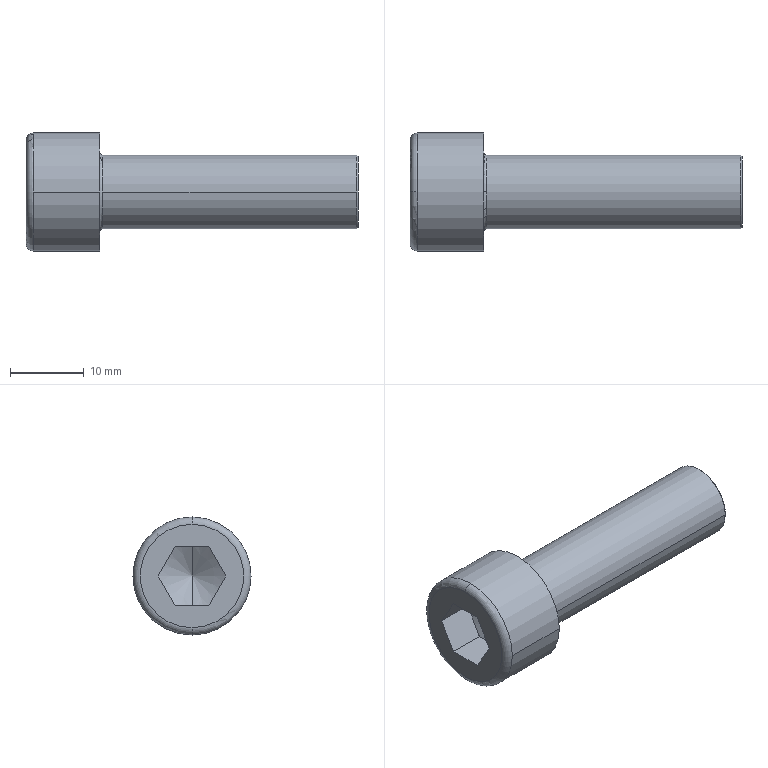Part | SolidWorks | features BaseBody 1 | 1 solid | 27 faces | box 45 x 16 x 16 mm | volume 4420 mm3 | plane 15 | cylinder 4 | cone 4 | torus 4 | commonest cylinder face diameters 10 x2 16 x2
STEP:
#1=CARTESIAN_POINT('',(34.8,0.,5.));
#2=VERTEX_POINT('',#1);
#3=CARTESIAN_POINT('',(34.8,5.,0.));
#4=VERTEX_POINT('',#3);
#5=CARTESIAN_POINT('',(34.8,0.,0.));
#6=DIRECTION('',(-1.,0.,0.));
#7=DIRECTION('',(0.,-1.,0.));
#8=AXIS2_PLACEMENT_3D('',#5,#6,#7);
#9=CIRCLE('',#8,5.);
#10=EDGE_CURVE('',#2,#4,#9,.T.);
#11=ORIENTED_EDGE('',*,*,#10,.T.);
#12=CARTESIAN_POINT('',(0.4,5.,0.));
#13=VERTEX_POINT('',#12);
#14=CARTESIAN_POINT('',(-2.359,5.,0.));
#15=DIRECTION('',(-1.,0.,0.));
#16=VECTOR('',#15,1000.);
#17=LINE('',#14,#16);
#18=EDGE_CURVE('',#4,#13,#17,.T.);
#19=ORIENTED_EDGE('',*,*,#18,.T.);
#20=CARTESIAN_POINT('',(0.4,0.,5.));
#21=VERTEX_POINT('',#20);
#22=CARTESIAN_POINT('',(0.4,0.,0.));
#23=DIRECTION('',(1.,0.,0.));
#24=DIRECTION('',(0.,-1.,0.));
#25=AXIS2_PLACEMENT_3D('',#22,#23,#24);
#26=CIRCLE('',#25,5.);
#27=EDGE_CURVE('',#13,#21,#26,.T.);
#28=ORIENTED_EDGE('',*,*,#27,.T.);
#29=CARTESIAN_POINT('',(0.4,-5.,0.));
#30=VERTEX_POINT('',#29);
#31=CARTESIAN_POINT('',(0.4,0.,0.));
#32=DIRECTION('',(1.,0.,0.));
#33=DIRECTION('',(0.,-1.,0.));
#34=AXIS2_PLACEMENT_3D('',#31,#32,#33);
#35=CIRCLE('',#34,5.);
#36=EDGE_CURVE('',#21,#30,#35,.T.);
#37=ORIENTED_EDGE('',*,*,#36,.T.);
#38=CARTESIAN_POINT('',(34.8,-5.,0.));
#39=VERTEX_POINT('',#38);
#40=CARTESIAN_POINT('',(-2.359,-5.,0.));
#41=DIRECTION('',(-1.,0.,0.));
#42=VECTOR('',#41,1000.);
#43=LINE('',#40,#42);
#44=EDGE_CURVE('',#39,#30,#43,.T.);
#45=ORIENTED_EDGE('',*,*,#44,.F.);
#46=CARTESIAN_POINT('',(34.8,0.,0.));
#47=DIRECTION('',(-1.,0.,0.));
#48=DIRECTION('',(0.,-1.,0.));
#49=AXIS2_PLACEMENT_3D('',#46,#47,#48);
#50=CIRCLE('',#49,5.);
#51=EDGE_CURVE('',#39,#2,#50,.T.);
#52=ORIENTED_EDGE('',*,*,#51,.T.);
#53=EDGE_LOOP('',(#11,#19,#28,#37,#45,#52));
#54=FACE_OUTER_BOUND('',#53,.T.);
#55=CARTESIAN_POINT('',(-2.359,0.,0.));
#56=DIRECTION('',(-1.,0.,0.));
#57=DIRECTION('',(0.,-1.,0.));
#58=AXIS2_PLACEMENT_3D('',#55,#56,#57);
#59=CYLINDRICAL_SURFACE('',#58,5.);
#60=ADVANCED_FACE('',(#54),#59,.T.);
#61=CARTESIAN_POINT('',(35.,0.,4.8));
#62=VERTEX_POINT('',#61);
#63=CARTESIAN_POINT('',(35.,0.,-4.8));
#64=VERTEX_POINT('',#63);
#65=CARTESIAN_POINT('',(35.,0.,0.));
#66=DIRECTION('',(-1.,0.,0.));
#67=DIRECTION('',(0.,0.,1.));
#68=AXIS2_PLACEMENT_3D('',#65,#66,#67);
#69=CIRCLE('',#68,4.8);
#70=EDGE_CURVE('',#62,#64,#69,.T.);
#71=ORIENTED_EDGE('',*,*,#70,.T.);
#72=CARTESIAN_POINT('',(34.8,0.,-5.));
#73=VERTEX_POINT('',#72);
#74=CARTESIAN_POINT('',(34.8,0.,-5.));
#75=DIRECTION('',(-0.7071,0.,-0.7071));
#76=VECTOR('',#75,1000.);
#77=LINE('',#74,#76);
#78=EDGE_CURVE('',#64,#73,#77,.T.);
#79=ORIENTED_EDGE('',*,*,#78,.T.);
#80=CARTESIAN_POINT('',(34.8,0.,0.));
#81=DIRECTION('',(-1.,0.,0.));
#82=DIRECTION('',(0.,-1.,0.));
#83=AXIS2_PLACEMENT_3D('',#80,#81,#82);
#84=CIRCLE('',#83,5.);
#85=EDGE_CURVE('',#4,#73,#84,.T.);
#86=ORIENTED_EDGE('',*,*,#85,.F.);
#87=ORIENTED_EDGE('',*,*,#10,.F.);
#88=CARTESIAN_POINT('',(34.8,0.,5.));
#89=DIRECTION('',(-0.7071,0.,0.7071));
#90=VECTOR('',#89,1000.);
#91=LINE('',#88,#90);
#92=EDGE_CURVE('',#62,#2,#91,.T.);
#93=ORIENTED_EDGE('',*,*,#92,.F.);
#94=EDGE_LOOP('',(#71,#79,#86,#87,#93));
#95=FACE_OUTER_BOUND('',#94,.T.);
#96=CARTESIAN_POINT('',(34.8,0.,0.));
#97=DIRECTION('',(-1.,0.,0.));
#98=DIRECTION('',(0.,0.,1.));
#99=AXIS2_PLACEMENT_3D('',#96,#97,#98);
#100=CONICAL_SURFACE('',#99,5.,0.7854);
#101=ADVANCED_FACE('',(#95),#100,.T.);
#102=CARTESIAN_POINT('',(0.,0.,-5.4));
#103=VERTEX_POINT('',#102);
#104=CARTESIAN_POINT('',(0.,0.,5.4));
#105=VERTEX_POINT('',#104);
#106=CARTESIAN_POINT('',(0.,0.,0.));
#107=DIRECTION('',(-1.,0.,0.));
#108=DIRECTION('',(0.,0.,1.));
#109=AXIS2_PLACEMENT_3D('',#106,#107,#108);
#110=CIRCLE('',#109,5.4);
#111=EDGE_CURVE('',#103,#105,#110,.T.);
#112=ORIENTED_EDGE('',*,*,#111,.F.);
#113=CARTESIAN_POINT('',(0.4,0.,-5.));
#114=VERTEX_POINT('',#113);
#115=CARTESIAN_POINT('',(0.4,0.,-5.4));
#116=DIRECTION('',(0.,1.,0.));
#117=DIRECTION('',(0.,0.,1.));
#118=AXIS2_PLACEMENT_3D('',#115,#116,#117);
#119=CIRCLE('',#118,0.4);
#120=EDGE_CURVE('',#103,#114,#119,.T.);
#121=ORIENTED_EDGE('',*,*,#120,.T.);
#122=CARTESIAN_POINT('',(0.4,0.,0.));
#123=DIRECTION('',(1.,0.,0.));
#124=DIRECTION('',(0.,-1.,0.));
#125=AXIS2_PLACEMENT_3D('',#122,#123,#124);
#126=CIRCLE('',#125,5.);
#127=EDGE_CURVE('',#30,#114,#126,.T.);
#128=ORIENTED_EDGE('',*,*,#127,.F.);
#129=ORIENTED_EDGE('',*,*,#36,.F.);
#130=CARTESIAN_POINT('',(0.4,0.,5.4));
#131=DIRECTION('',(0.,-1.,0.));
#132=DIRECTION('',(1.,0.,0.));
#133=AXIS2_PLACEMENT_3D('',#130,#131,#132);
#134=CIRCLE('',#133,0.4);
#135=EDGE_CURVE('',#105,#21,#134,.T.);
#136=ORIENTED_EDGE('',*,*,#135,.F.);
#137=EDGE_LOOP('',(#112,#121,#128,#129,#136));
#138=FACE_OUTER_BOUND('',#137,.T.);
#139=CARTESIAN_POINT('',(0.4,0.,0.));
#140=DIRECTION('',(-1.,0.,0.));
#141=DIRECTION('',(0.,0.,1.));
#142=AXIS2_PLACEMENT_3D('',#139,#140,#141);
#143=TOROIDAL_SURFACE('',#142,5.4,0.4);
#144=ADVANCED_FACE('',(#138),#143,.F.);
#145=CARTESIAN_POINT('',(0.,-8.,0.));
#146=VERTEX_POINT('',#145);
#147=CARTESIAN_POINT('',(0.,8.,0.));
#148=VERTEX_POINT('',#147);
#149=CARTESIAN_POINT('',(0.,0.,0.));
#150=DIRECTION('',(-1.,0.,0.));
#151=DIRECTION('',(0.,-1.,0.));
#152=AXIS2_PLACEMENT_3D('',#149,#150,#151);
#153=CIRCLE('',#152,8.);
#154=EDGE_CURVE('',#146,#148,#153,.T.);
#155=ORIENTED_EDGE('',*,*,#154,.T.);
#156=CARTESIAN_POINT('',(-9.,8.,0.));
#157=VERTEX_POINT('',#156);
#158=CARTESIAN_POINT('',(-2.359,8.,0.));
#159=DIRECTION('',(-1.,0.,0.));
#160=VECTOR('',#159,1000.);
#161=LINE('',#158,#160);
#162=EDGE_CURVE('',#148,#157,#161,.T.);
#163=ORIENTED_EDGE('',*,*,#162,.T.);
#164=CARTESIAN_POINT('',(-9.,0.,8.));
#165=VERTEX_POINT('',#164);
#166=CARTESIAN_POINT('',(-9.,0.,0.));
#167=DIRECTION('',(1.,0.,0.));
#168=DIRECTION('',(0.,-1.,0.));
#169=AXIS2_PLACEMENT_3D('',#166,#167,#168);
#170=CIRCLE('',#169,8.);
#171=EDGE_CURVE('',#157,#165,#170,.T.);
#172=ORIENTED_EDGE('',*,*,#171,.T.);
#173=CARTESIAN_POINT('',(-9.,-8.,0.));
#174=VERTEX_POINT('',#173);
#175=CARTESIAN_POINT('',(-9.,0.,0.));
#176=DIRECTION('',(1.,0.,0.));
#177=DIRECTION('',(0.,-1.,0.));
#178=AXIS2_PLACEMENT_3D('',#175,#176,#177);
#179=CIRCLE('',#178,8.);
#180=EDGE_CURVE('',#165,#174,#179,.T.);
#181=ORIENTED_EDGE('',*,*,#180,.T.);
#182=CARTESIAN_POINT('',(-2.359,-8.,0.));
#183=DIRECTION('',(-1.,0.,0.));
#184=VECTOR('',#183,1000.);
#185=LINE('',#182,#184);
#186=EDGE_CURVE('',#146,#174,#185,.T.);
#187=ORIENTED_EDGE('',*,*,#186,.F.);
#188=EDGE_LOOP('',(#155,#163,#172,#181,#187));
#189=FACE_OUTER_BOUND('',#188,.T.);
#190=CARTESIAN_POINT('',(-2.359,0.,0.));
#191=DIRECTION('',(-1.,0.,0.));
#192=DIRECTION('',(0.,-1.,0.));
#193=AXIS2_PLACEMENT_3D('',#190,#191,#192);
#194=CYLINDRICAL_SURFACE('',#193,8.);
#195=ADVANCED_FACE('',(#189),#194,.T.);
#196=CARTESIAN_POINT('',(-9.,0.,-8.));
#197=VERTEX_POINT('',#196);
#198=CARTESIAN_POINT('',(-9.,0.,0.));
#199=DIRECTION('',(1.,0.,0.));
#200=DIRECTION('',(0.,-1.,0.));
#201=AXIS2_PLACEMENT_3D('',#198,#199,#200);
#202=CIRCLE('',#201,8.);
#203=EDGE_CURVE('',#197,#157,#202,.T.);
#204=ORIENTED_EDGE('',*,*,#203,.F.);
#205=CARTESIAN_POINT('',(-10.,0.,-7.));
#206=VERTEX_POINT('',#205);
#207=CARTESIAN_POINT('',(-9.,0.,-7.));
#208=DIRECTION('',(0.,1.,0.));
#209=DIRECTION('',(0.,0.,1.));
#210=AXIS2_PLACEMENT_3D('',#207,#208,#209);
#211=CIRCLE('',#210,1.);
#212=EDGE_CURVE('',#197,#206,#211,.T.);
#213=ORIENTED_EDGE('',*,*,#212,.T.);
#214=CARTESIAN_POINT('',(-10.,0.,7.));
#215=VERTEX_POINT('',#214);
#216=CARTESIAN_POINT('',(-10.,0.,0.));
#217=DIRECTION('',(1.,0.,0.));
#218=DIRECTION('',(0.,0.,1.));
#219=AXIS2_PLACEMENT_3D('',#216,#217,#218);
#220=CIRCLE('',#219,7.);
#221=EDGE_CURVE('',#206,#215,#220,.T.);
#222=ORIENTED_EDGE('',*,*,#221,.T.);
#223=CARTESIAN_POINT('',(-9.,0.,7.));
#224=DIRECTION('',(0.,-1.,0.));
#225=DIRECTION('',(0.,0.,-1.));
#226=AXIS2_PLACEMENT_3D('',#223,#224,#225);
#227=CIRCLE('',#226,1.);
#228=EDGE_CURVE('',#165,#215,#227,.T.);
#229=ORIENTED_EDGE('',*,*,#228,.F.);
#230=ORIENTED_EDGE('',*,*,#171,.F.);
#231=EDGE_LOOP('',(#204,#213,#222,#229,#230));
#232=FACE_OUTER_BOUND('',#231,.T.);
#233=CARTESIAN_POINT('',(-9.,0.,0.));
#234=DIRECTION('',(-1.,0.,0.));
#235=DIRECTION('',(0.,0.,1.));
#236=AXIS2_PLACEMENT_3D('',#233,#234,#235);
#237=TOROIDAL_SURFACE('',#236,7.,1.);
#238=ADVANCED_FACE('',(#232),#237,.T.);
#239=CARTESIAN_POINT('',(-2.359,0.,0.));
#240=VERTEX_POINT('',#239);
#241=CARTESIAN_POINT('',(-5.,0.,4.574));
#242=VERTEX_POINT('',#241);
#243=CARTESIAN_POINT('',(-5.,0.,4.575));
#244=DIRECTION('',(-0.5,0.,0.866));
#245=VECTOR('',#244,1000.);
#246=LINE('',#243,#245);
#247=EDGE_CURVE('',#240,#242,#246,.T.);
#248=ORIENTED_EDGE('',*,*,#247,.F.);
#249=CARTESIAN_POINT('',(-5.,0.,-4.575));
#250=VERTEX_POINT('',#249);
#251=CARTESIAN_POINT('',(-5.,0.,-4.575));
#252=DIRECTION('',(-0.5,0.,-0.866));
#253=VECTOR('',#252,1000.);
#254=LINE('',#251,#253);
#255=EDGE_CURVE('',#240,#250,#254,.T.);
#256=ORIENTED_EDGE('',*,*,#255,.T.);
#257=CARTESIAN_POINT('',(-5.,-2.287,-3.962));
#258=VERTEX_POINT('',#257);
#259=CARTESIAN_POINT('',(-5.,0.,0.));
#260=DIRECTION('',(-1.,0.,0.));
#261=DIRECTION('',(0.,0.,1.));
#262=AXIS2_PLACEMENT_3D('',#259,#260,#261);
#263=CIRCLE('',#262,4.574);
#264=EDGE_CURVE('',#250,#258,#263,.T.);
#265=ORIENTED_EDGE('',*,*,#264,.T.);
#266=CARTESIAN_POINT('',(-5.,-4.575,0.));
#267=VERTEX_POINT('',#266);
#268=CARTESIAN_POINT('',(-5.,0.,0.));
#269=DIRECTION('',(-1.,0.,0.));
#270=DIRECTION('',(0.,0.,1.));
#271=AXIS2_PLACEMENT_3D('',#268,#269,#270);
#272=CIRCLE('',#271,4.575);
#273=EDGE_CURVE('',#258,#267,#272,.T.);
#274=ORIENTED_EDGE('',*,*,#273,.T.);
#275=CARTESIAN_POINT('',(-5.,-2.287,3.962));
#276=VERTEX_POINT('',#275);
#277=CARTESIAN_POINT('',(-5.,0.,0.));
#278=DIRECTION('',(-1.,0.,0.));
#279=DIRECTION('',(0.,0.,1.));
#280=AXIS2_PLACEMENT_3D('',#277,#278,#279);
#281=CIRCLE('',#280,4.574);
#282=EDGE_CURVE('',#267,#276,#281,.T.);
#283=ORIENTED_EDGE('',*,*,#282,.T.);
#284=CARTESIAN_POINT('',(-5.,0.,0.));
#285=DIRECTION('',(-1.,0.,0.));
#286=DIRECTION('',(0.,0.,1.));
#287=AXIS2_PLACEMENT_3D('',#284,#285,#286);
#288=CIRCLE('',#287,4.574);
#289=EDGE_CURVE('',#276,#242,#288,.T.);
#290=ORIENTED_EDGE('',*,*,#289,.T.);
#291=EDGE_LOOP('',(#248,#256,#265,#274,#283,#290));
#292=FACE_OUTER_BOUND('',#291,.T.);
#293=CARTESIAN_POINT('',(-5.,0.,0.));
#294=DIRECTION('',(-1.,0.,0.));
#295=DIRECTION('',(0.,0.,1.));
#296=AXIS2_PLACEMENT_3D('',#293,#294,#295);
#297=CONICAL_SURFACE('',#296,4.575,1.047);
#298=ADVANCED_FACE('',(#292),#297,.F.);
#299=ORIENTED_EDGE('',*,*,#18,.F.);
#300=ORIENTED_EDGE('',*,*,#85,.T.);
#301=CARTESIAN_POINT('',(34.8,0.,0.));
#302=DIRECTION('',(-1.,0.,0.));
#303=DIRECTION('',(0.,-1.,0.));
#304=AXIS2_PLACEMENT_3D('',#301,#302,#303);
#305=CIRCLE('',#304,5.);
#306=EDGE_CURVE('',#73,#39,#305,.T.);
#307=ORIENTED_EDGE('',*,*,#306,.T.);
#308=ORIENTED_EDGE('',*,*,#44,.T.);
#309=ORIENTED_EDGE('',*,*,#127,.T.);
#310=CARTESIAN_POINT('',(0.4,0.,0.));
#311=DIRECTION('',(1.,0.,0.));
#312=DIRECTION('',(0.,-1.,0.));
#313=AXIS2_PLACEMENT_3D('',#310,#311,#312);
#314=CIRCLE('',#313,5.);
#315=EDGE_CURVE('',#114,#13,#314,.T.);
#316=ORIENTED_EDGE('',*,*,#315,.T.);
#317=EDGE_LOOP('',(#299,#300,#307,#308,#309,#316));
#318=FACE_OUTER_BOUND('',#317,.T.);
#319=CARTESIAN_POINT('',(-2.359,0.,0.));
#320=DIRECTION('',(-1.,0.,0.));
#321=DIRECTION('',(0.,-1.,0.));
#322=AXIS2_PLACEMENT_3D('',#319,#320,#321);
#323=CYLINDRICAL_SURFACE('',#322,5.);
#324=ADVANCED_FACE('',(#318),#323,.T.);
#325=ORIENTED_EDGE('',*,*,#78,.F.);
#326=CARTESIAN_POINT('',(35.,0.,0.));
#327=DIRECTION('',(-1.,0.,0.));
#328=DIRECTION('',(0.,0.,1.));
#329=AXIS2_PLACEMENT_3D('',#326,#327,#328);
#330=CIRCLE('',#329,4.8);
#331=EDGE_CURVE('',#64,#62,#330,.T.);
#332=ORIENTED_EDGE('',*,*,#331,.T.);
#333=ORIENTED_EDGE('',*,*,#92,.T.);
#334=ORIENTED_EDGE('',*,*,#51,.F.);
#335=ORIENTED_EDGE('',*,*,#306,.F.);
#336=EDGE_LOOP('',(#325,#332,#333,#334,#335));
#337=FACE_OUTER_BOUND('',#336,.T.);
#338=CARTESIAN_POINT('',(34.8,0.,0.));
#339=DIRECTION('',(-1.,0.,0.));
#340=DIRECTION('',(0.,0.,1.));
#341=AXIS2_PLACEMENT_3D('',#338,#339,#340);
#342=CONICAL_SURFACE('',#341,5.,0.7854);
#343=ADVANCED_FACE('',(#337),#342,.T.);
#344=ORIENTED_EDGE('',*,*,#120,.F.);
#345=CARTESIAN_POINT('',(0.,0.,0.));
#346=DIRECTION('',(-1.,0.,0.));
#347=DIRECTION('',(0.,0.,1.));
#348=AXIS2_PLACEMENT_3D('',#345,#346,#347);
#349=CIRCLE('',#348,5.4);
#350=EDGE_CURVE('',#105,#103,#349,.T.);
#351=ORIENTED_EDGE('',*,*,#350,.F.);
#352=ORIENTED_EDGE('',*,*,#135,.T.);
#353=ORIENTED_EDGE('',*,*,#27,.F.);
#354=ORIENTED_EDGE('',*,*,#315,.F.);
#355=EDGE_LOOP('',(#344,#351,#352,#353,#354));
#356=FACE_OUTER_BOUND('',#355,.T.);
#357=CARTESIAN_POINT('',(0.4,0.,0.));
#358=DIRECTION('',(-1.,0.,0.));
#359=DIRECTION('',(0.,0.,1.));
#360=AXIS2_PLACEMENT_3D('',#357,#358,#359);
#361=TOROIDAL_SURFACE('',#360,5.4,0.4);
#362=ADVANCED_FACE('',(#356),#361,.F.);
#363=ORIENTED_EDGE('',*,*,#70,.F.);
#364=ORIENTED_EDGE('',*,*,#331,.F.);
#365=EDGE_LOOP('',(#363,#364));
#366=FACE_OUTER_BOUND('',#365,.T.);
#367=CARTESIAN_POINT('',(35.,4.8,0.));
#368=DIRECTION('',(-1.,0.,0.));
#369=DIRECTION('',(0.,-1.,0.));
#370=AXIS2_PLACEMENT_3D('',#367,#368,#369);
#371=PLANE('',#370);
#372=ADVANCED_FACE('',(#366),#371,.F.);
#373=ORIENTED_EDGE('',*,*,#154,.F.);
#374=CARTESIAN_POINT('',(0.,0.,0.));
#375=DIRECTION('',(-1.,0.,0.));
#376=DIRECTION('',(0.,-1.,0.));
#377=AXIS2_PLACEMENT_3D('',#374,#375,#376);
#378=CIRCLE('',#377,8.);
#379=EDGE_CURVE('',#148,#146,#378,.T.);
#380=ORIENTED_EDGE('',*,*,#379,.F.);
#381=EDGE_LOOP('',(#373,#380));
#382=FACE_OUTER_BOUND('',#381,.T.);
#383=ORIENTED_EDGE('',*,*,#350,.T.);
#384=ORIENTED_EDGE('',*,*,#111,.T.);
#385=EDGE_LOOP('',(#383,#384));
#386=FACE_BOUND('',#385,.T.);
#387=CARTESIAN_POINT('',(0.,8.,0.));
#388=DIRECTION('',(-1.,0.,0.));
#389=DIRECTION('',(0.,-1.,0.));
#390=AXIS2_PLACEMENT_3D('',#387,#388,#389);
#391=PLANE('',#390);
#392=ADVANCED_FACE('',(#382,#386),#391,.F.);
#393=ORIENTED_EDGE('',*,*,#162,.F.);
#394=ORIENTED_EDGE('',*,*,#379,.T.);
#395=ORIENTED_EDGE('',*,*,#186,.T.);
#396=CARTESIAN_POINT('',(-9.,0.,0.));
#397=DIRECTION('',(1.,0.,0.));
#398=DIRECTION('',(0.,-1.,0.));
#399=AXIS2_PLACEMENT_3D('',#396,#397,#398);
#400=CIRCLE('',#399,8.);
#401=EDGE_CURVE('',#174,#197,#400,.T.);
#402=ORIENTED_EDGE('',*,*,#401,.T.);
#403=ORIENTED_EDGE('',*,*,#203,.T.);
#404=EDGE_LOOP('',(#393,#394,#395,#402,#403));
#405=FACE_OUTER_BOUND('',#404,.T.);
#406=CARTESIAN_POINT('',(-2.359,0.,0.));
#407=DIRECTION('',(-1.,0.,0.));
#408=DIRECTION('',(0.,-1.,0.));
#409=AXIS2_PLACEMENT_3D('',#406,#407,#408);
#410=CYLINDRICAL_SURFACE('',#409,8.);
#411=ADVANCED_FACE('',(#405),#410,.T.);
#412=ORIENTED_EDGE('',*,*,#212,.F.);
#413=ORIENTED_EDGE('',*,*,#401,.F.);
#414=ORIENTED_EDGE('',*,*,#180,.F.);
#415=ORIENTED_EDGE('',*,*,#228,.T.);
#416=CARTESIAN_POINT('',(-10.,0.,0.));
#417=DIRECTION('',(1.,0.,0.));
#418=DIRECTION('',(0.,0.,1.));
#419=AXIS2_PLACEMENT_3D('',#416,#417,#418);
#420=CIRCLE('',#419,7.);
#421=EDGE_CURVE('',#215,#206,#420,.T.);
#422=ORIENTED_EDGE('',*,*,#421,.T.);
#423=EDGE_LOOP('',(#412,#413,#414,#415,#422));
#424=FACE_OUTER_BOUND('',#423,.T.);
#425=CARTESIAN_POINT('',(-9.,0.,0.));
#426=DIRECTION('',(-1.,0.,0.));
#427=DIRECTION('',(0.,0.,1.));
#428=AXIS2_PLACEMENT_3D('',#425,#426,#427);
#429=TOROIDAL_SURFACE('',#428,7.,1.);
#430=ADVANCED_FACE('',(#424),#429,.T.);
#431=CARTESIAN_POINT('',(-10.,2.287,-3.962));
#432=VERTEX_POINT('',#431);
#433=CARTESIAN_POINT('',(-10.,-2.287,-3.962));
#434=VERTEX_POINT('',#433);
#435=CARTESIAN_POINT('',(-10.,4.574,-3.962));
#436=DIRECTION('',(0.,-1.,0.));
#437=VECTOR('',#436,1000.);
#438=LINE('',#435,#437);
#439=EDGE_CURVE('',#432,#434,#438,.T.);
#440=ORIENTED_EDGE('',*,*,#439,.F.);
#441=CARTESIAN_POINT('',(-10.,4.575,0.));
#442=VERTEX_POINT('',#441);
#443=CARTESIAN_POINT('',(-10.,4.574,0.));
#444=DIRECTION('',(0.,-0.5,-0.866));
#445=VECTOR('',#444,1000.);
#446=LINE('',#443,#445);
#447=EDGE_CURVE('',#442,#432,#446,.T.);
#448=ORIENTED_EDGE('',*,*,#447,.F.);
#449=CARTESIAN_POINT('',(-10.,2.287,3.962));
#450=VERTEX_POINT('',#449);
#451=CARTESIAN_POINT('',(-10.,2.287,3.962));
#452=DIRECTION('',(0.,0.5,-0.866));
#453=VECTOR('',#452,1000.);
#454=LINE('',#451,#453);
#455=EDGE_CURVE('',#450,#442,#454,.T.);
#456=ORIENTED_EDGE('',*,*,#455,.F.);
#457=CARTESIAN_POINT('',(-10.,-2.287,3.962));
#458=VERTEX_POINT('',#457);
#459=CARTESIAN_POINT('',(-10.,4.574,3.962));
#460=DIRECTION('',(0.,1.,0.));
#461=VECTOR('',#460,1000.);
#462=LINE('',#459,#461);
#463=EDGE_CURVE('',#458,#450,#462,.T.);
#464=ORIENTED_EDGE('',*,*,#463,.F.);
#465=CARTESIAN_POINT('',(-10.,-4.575,0.));
#466=VERTEX_POINT('',#465);
#467=CARTESIAN_POINT('',(-10.,-4.574,0.));
#468=DIRECTION('',(0.,0.5,0.866));
#469=VECTOR('',#468,1000.);
#470=LINE('',#467,#469);
#471=EDGE_CURVE('',#466,#458,#470,.T.);
#472=ORIENTED_EDGE('',*,*,#471,.F.);
#473=CARTESIAN_POINT('',(-10.,-2.287,-3.962));
#474=DIRECTION('',(0.,-0.5,0.866));
#475=VECTOR('',#474,1000.);
#476=LINE('',#473,#475);
#477=EDGE_CURVE('',#434,#466,#476,.T.);
#478=ORIENTED_EDGE('',*,*,#477,.F.);
#479=EDGE_LOOP('',(#440,#448,#456,#464,#472,#478));
#480=FACE_BOUND('',#479,.T.);
#481=ORIENTED_EDGE('',*,*,#421,.F.);
#482=ORIENTED_EDGE('',*,*,#221,.F.);
#483=EDGE_LOOP('',(#481,#482));
#484=FACE_OUTER_BOUND('',#483,.T.);
#485=CARTESIAN_POINT('',(-10.,4.574,0.));
#486=DIRECTION('',(1.,0.,0.));
#487=DIRECTION('',(0.,1.,0.));
#488=AXIS2_PLACEMENT_3D('',#485,#486,#487);
#489=PLANE('',#488);
#490=ADVANCED_FACE('',(#480,#484),#489,.F.);
#491=CARTESIAN_POINT('',(-5.,-2.287,-3.962));
#492=DIRECTION('',(0.,-0.5,0.866));
#493=VECTOR('',#492,1000.);
#494=LINE('',#491,#493);
#495=EDGE_CURVE('',#258,#267,#494,.T.);
#496=ORIENTED_EDGE('',*,*,#495,.F.);
#497=CARTESIAN_POINT('',(-5.,-2.287,-3.962));
#498=DIRECTION('',(1.,0.,0.));
#499=VECTOR('',#498,1000.);
#500=LINE('',#497,#499);
#501=EDGE_CURVE('',#434,#258,#500,.T.);
#502=ORIENTED_EDGE('',*,*,#501,.F.);
#503=ORIENTED_EDGE('',*,*,#477,.T.);
#504=CARTESIAN_POINT('',(-5.,-4.575,0.));
#505=DIRECTION('',(-1.,0.,0.));
#506=VECTOR('',#505,1000.);
#507=LINE('',#504,#506);
#508=EDGE_CURVE('',#267,#466,#507,.T.);
#509=ORIENTED_EDGE('',*,*,#508,.F.);
#510=EDGE_LOOP('',(#496,#502,#503,#509));
#511=FACE_OUTER_BOUND('',#510,.T.);
#512=CARTESIAN_POINT('',(-5.,-2.287,-3.962));
#513=DIRECTION('',(0.,-0.866,-0.5));
#514=DIRECTION('',(0.,0.5,-0.866));
#515=AXIS2_PLACEMENT_3D('',#512,#513,#514);
#516=PLANE('',#515);
#517=ADVANCED_FACE('',(#511),#516,.F.);
#518=CARTESIAN_POINT('',(-5.,2.287,-3.962));
#519=VERTEX_POINT('',#518);
#520=CARTESIAN_POINT('',(-5.,2.287,-3.962));
#521=DIRECTION('',(0.,-1.,0.));
#522=VECTOR('',#521,1000.);
#523=LINE('',#520,#522);
#524=EDGE_CURVE('',#519,#258,#523,.T.);
#525=ORIENTED_EDGE('',*,*,#524,.F.);
#526=CARTESIAN_POINT('',(-5.,2.287,-3.962));
#527=DIRECTION('',(1.,0.,0.));
#528=VECTOR('',#527,1000.);
#529=LINE('',#526,#528);
#530=EDGE_CURVE('',#432,#519,#529,.T.);
#531=ORIENTED_EDGE('',*,*,#530,.F.);
#532=ORIENTED_EDGE('',*,*,#439,.T.);
#533=ORIENTED_EDGE('',*,*,#501,.T.);
#534=EDGE_LOOP('',(#525,#531,#532,#533));
#535=FACE_OUTER_BOUND('',#534,.T.);
#536=CARTESIAN_POINT('',(-5.,2.287,-3.962));
#537=DIRECTION('',(0.,0.,-1.));
#538=DIRECTION('',(0.,1.,0.));
#539=AXIS2_PLACEMENT_3D('',#536,#537,#538);
#540=PLANE('',#539);
#541=ADVANCED_FACE('',(#535),#540,.F.);
#542=CARTESIAN_POINT('',(-5.,4.574,0.));
#543=VERTEX_POINT('',#542);
#544=CARTESIAN_POINT('',(-5.,4.574,0.));
#545=DIRECTION('',(0.,-0.5,-0.866));
#546=VECTOR('',#545,1000.);
#547=LINE('',#544,#546);
#548=EDGE_CURVE('',#543,#519,#547,.T.);
#549=ORIENTED_EDGE('',*,*,#548,.F.);
#550=CARTESIAN_POINT('',(-5.,4.574,0.));
#551=DIRECTION('',(1.,0.,0.));
#552=VECTOR('',#551,1000.);
#553=LINE('',#550,#552);
#554=EDGE_CURVE('',#442,#543,#553,.T.);
#555=ORIENTED_EDGE('',*,*,#554,.F.);
#556=ORIENTED_EDGE('',*,*,#447,.T.);
#557=ORIENTED_EDGE('',*,*,#530,.T.);
#558=EDGE_LOOP('',(#549,#555,#556,#557));
#559=FACE_OUTER_BOUND('',#558,.T.);
#560=CARTESIAN_POINT('',(-5.,4.574,0.));
#561=DIRECTION('',(0.,0.866,-0.5));
#562=DIRECTION('',(0.,0.5,0.866));
#563=AXIS2_PLACEMENT_3D('',#560,#561,#562);
#564=PLANE('',#563);
#565=ADVANCED_FACE('',(#559),#564,.F.);
#566=CARTESIAN_POINT('',(-5.,2.287,3.962));
#567=VERTEX_POINT('',#566);
#568=CARTESIAN_POINT('',(-5.,2.287,3.962));
#569=DIRECTION('',(0.,0.5,-0.866));
#570=VECTOR('',#569,1000.);
#571=LINE('',#568,#570);
#572=EDGE_CURVE('',#567,#543,#571,.T.);
#573=ORIENTED_EDGE('',*,*,#572,.F.);
#574=CARTESIAN_POINT('',(-5.,2.287,3.962));
#575=DIRECTION('',(1.,0.,0.));
#576=VECTOR('',#575,1000.);
#577=LINE('',#574,#576);
#578=EDGE_CURVE('',#450,#567,#577,.T.);
#579=ORIENTED_EDGE('',*,*,#578,.F.);
#580=ORIENTED_EDGE('',*,*,#455,.T.);
#581=ORIENTED_EDGE('',*,*,#554,.T.);
#582=EDGE_LOOP('',(#573,#579,#580,#581));
#583=FACE_OUTER_BOUND('',#582,.T.);
#584=CARTESIAN_POINT('',(-5.,2.287,3.962));
#585=DIRECTION('',(0.,0.866,0.5));
#586=DIRECTION('',(0.,-0.5,0.866));
#587=AXIS2_PLACEMENT_3D('',#584,#585,#586);
#588=PLANE('',#587);
#589=ADVANCED_FACE('',(#583),#588,.F.);
#590=CARTESIAN_POINT('',(-5.,-2.287,3.962));
#591=DIRECTION('',(0.,1.,0.));
#592=VECTOR('',#591,1000.);
#593=LINE('',#590,#592);
#594=EDGE_CURVE('',#276,#567,#593,.T.);
#595=ORIENTED_EDGE('',*,*,#594,.F.);
#596=CARTESIAN_POINT('',(-5.,-2.287,3.962));
#597=DIRECTION('',(1.,0.,0.));
#598=VECTOR('',#597,1000.);
#599=LINE('',#596,#598);
#600=EDGE_CURVE('',#458,#276,#599,.T.);
#601=ORIENTED_EDGE('',*,*,#600,.F.);
#602=ORIENTED_EDGE('',*,*,#463,.T.);
#603=ORIENTED_EDGE('',*,*,#578,.T.);
#604=EDGE_LOOP('',(#595,#601,#602,#603));
#605=FACE_OUTER_BOUND('',#604,.T.);
#606=CARTESIAN_POINT('',(-5.,-2.287,3.962));
#607=DIRECTION('',(0.,0.,1.));
#608=DIRECTION('',(1.,0.,0.));
#609=AXIS2_PLACEMENT_3D('',#606,#607,#608);
#610=PLANE('',#609);
#611=ADVANCED_FACE('',(#605),#610,.F.);
#612=CARTESIAN_POINT('',(-5.,-4.574,0.));
#613=DIRECTION('',(0.,0.5,0.866));
#614=VECTOR('',#613,1000.);
#615=LINE('',#612,#614);
#616=EDGE_CURVE('',#267,#276,#615,.T.);
#617=ORIENTED_EDGE('',*,*,#616,.F.);
#618=ORIENTED_EDGE('',*,*,#508,.T.);
#619=ORIENTED_EDGE('',*,*,#471,.T.);
#620=ORIENTED_EDGE('',*,*,#600,.T.);
#621=EDGE_LOOP('',(#617,#618,#619,#620));
#622=FACE_OUTER_BOUND('',#621,.T.);
#623=CARTESIAN_POINT('',(-5.,-4.574,0.));
#624=DIRECTION('',(0.,-0.866,0.5));
#625=DIRECTION('',(0.,-0.5,-0.866));
#626=AXIS2_PLACEMENT_3D('',#623,#624,#625);
#627=PLANE('',#626);
#628=ADVANCED_FACE('',(#622),#627,.F.);
#629=ORIENTED_EDGE('',*,*,#495,.T.);
#630=ORIENTED_EDGE('',*,*,#273,.F.);
#631=EDGE_LOOP('',(#629,#630));
#632=FACE_OUTER_BOUND('',#631,.T.);
#633=CARTESIAN_POINT('',(-5.,0.,0.));
#634=DIRECTION('',(-1.,0.,0.));
#635=DIRECTION('',(0.,-1.,0.));
#636=AXIS2_PLACEMENT_3D('',#633,#634,#635);
#637=PLANE('',#636);
#638=ADVANCED_FACE('',(#632),#637,.F.);
#639=ORIENTED_EDGE('',*,*,#524,.T.);
#640=ORIENTED_EDGE('',*,*,#264,.F.);
#641=CARTESIAN_POINT('',(-5.,0.,0.));
#642=DIRECTION('',(-1.,0.,0.));
#643=DIRECTION('',(0.,0.,1.));
#644=AXIS2_PLACEMENT_3D('',#641,#642,#643);
#645=CIRCLE('',#644,4.574);
#646=EDGE_CURVE('',#519,#250,#645,.T.);
#647=ORIENTED_EDGE('',*,*,#646,.F.);
#648=EDGE_LOOP('',(#639,#640,#647));
#649=FACE_OUTER_BOUND('',#648,.T.);
#650=CARTESIAN_POINT('',(-5.,0.,0.));
#651=DIRECTION('',(-1.,0.,0.));
#652=DIRECTION('',(0.,-1.,0.));
#653=AXIS2_PLACEMENT_3D('',#650,#651,#652);
#654=PLANE('',#653);
#655=ADVANCED_FACE('',(#649),#654,.F.);
#656=ORIENTED_EDGE('',*,*,#548,.T.);
#657=CARTESIAN_POINT('',(-5.,0.,0.));
#658=DIRECTION('',(-1.,0.,0.));
#659=DIRECTION('',(0.,0.,1.));
#660=AXIS2_PLACEMENT_3D('',#657,#658,#659);
#661=CIRCLE('',#660,4.574);
#662=EDGE_CURVE('',#543,#519,#661,.T.);
#663=ORIENTED_EDGE('',*,*,#662,.F.);
#664=EDGE_LOOP('',(#656,#663));
#665=FACE_OUTER_BOUND('',#664,.T.);
#666=CARTESIAN_POINT('',(-5.,0.,0.));
#667=DIRECTION('',(-1.,0.,0.));
#668=DIRECTION('',(0.,-1.,0.));
#669=AXIS2_PLACEMENT_3D('',#666,#667,#668);
#670=PLANE('',#669);
#671=ADVANCED_FACE('',(#665),#670,.F.);
#672=ORIENTED_EDGE('',*,*,#572,.T.);
#673=CARTESIAN_POINT('',(-5.,0.,0.));
#674=DIRECTION('',(-1.,0.,0.));
#675=DIRECTION('',(0.,0.,1.));
#676=AXIS2_PLACEMENT_3D('',#673,#674,#675);
#677=CIRCLE('',#676,4.574);
#678=EDGE_CURVE('',#567,#543,#677,.T.);
#679=ORIENTED_EDGE('',*,*,#678,.F.);
#680=EDGE_LOOP('',(#672,#679));
#681=FACE_OUTER_BOUND('',#680,.T.);
#682=CARTESIAN_POINT('',(-5.,0.,0.));
#683=DIRECTION('',(-1.,0.,0.));
#684=DIRECTION('',(0.,-1.,0.));
#685=AXIS2_PLACEMENT_3D('',#682,#683,#684);
#686=PLANE('',#685);
#687=ADVANCED_FACE('',(#681),#686,.F.);
#688=ORIENTED_EDGE('',*,*,#594,.T.);
#689=CARTESIAN_POINT('',(-5.,0.,0.));
#690=DIRECTION('',(-1.,0.,0.));
#691=DIRECTION('',(0.,0.,1.));
#692=AXIS2_PLACEMENT_3D('',#689,#690,#691);
#693=CIRCLE('',#692,4.574);
#694=EDGE_CURVE('',#242,#567,#693,.T.);
#695=ORIENTED_EDGE('',*,*,#694,.F.);
#696=ORIENTED_EDGE('',*,*,#289,.F.);
#697=EDGE_LOOP('',(#688,#695,#696));
#698=FACE_OUTER_BOUND('',#697,.T.);
#699=CARTESIAN_POINT('',(-5.,0.,0.));
#700=DIRECTION('',(-1.,0.,0.));
#701=DIRECTION('',(0.,-1.,0.));
#702=AXIS2_PLACEMENT_3D('',#699,#700,#701);
#703=PLANE('',#702);
#704=ADVANCED_FACE('',(#698),#703,.F.);
#705=ORIENTED_EDGE('',*,*,#616,.T.);
#706=ORIENTED_EDGE('',*,*,#282,.F.);
#707=EDGE_LOOP('',(#705,#706));
#708=FACE_OUTER_BOUND('',#707,.T.);
#709=CARTESIAN_POINT('',(-5.,0.,0.));
#710=DIRECTION('',(-1.,0.,0.));
#711=DIRECTION('',(0.,-1.,0.));
#712=AXIS2_PLACEMENT_3D('',#709,#710,#711);
#713=PLANE('',#712);
#714=ADVANCED_FACE('',(#708),#713,.F.);
#715=ORIENTED_EDGE('',*,*,#255,.F.);
#716=ORIENTED_EDGE('',*,*,#247,.T.);
#717=ORIENTED_EDGE('',*,*,#694,.T.);
#718=ORIENTED_EDGE('',*,*,#678,.T.);
#719=ORIENTED_EDGE('',*,*,#662,.T.);
#720=ORIENTED_EDGE('',*,*,#646,.T.);
#721=EDGE_LOOP('',(#715,#716,#717,#718,#719,#720));
#722=FACE_OUTER_BOUND('',#721,.T.);
#723=CARTESIAN_POINT('',(-5.,0.,0.));
#724=DIRECTION('',(-1.,0.,0.));
#725=DIRECTION('',(0.,0.,1.));
#726=AXIS2_PLACEMENT_3D('',#723,#724,#725);
#727=CONICAL_SURFACE('',#726,4.575,1.047);
#728=ADVANCED_FACE('',(#722),#727,.F.);
#729=CLOSED_SHELL('',(#60,#101,#144,#195,#238,#298,#324,#343,#362,#372,#392,#411,#430,#490,#517,#541,#565,#589,#611,#628,#638,#655,#671,#687,#704,#714,#728));
#730=MANIFOLD_SOLID_BREP('',#729);
#731=CARTESIAN_POINT('',(0.,0.,0.));
#732=DIRECTION('',(0.,0.,1.));
#733=DIRECTION('',(1.,0.,0.));
#734=AXIS2_PLACEMENT_3D('',#731,#732,#733);
#735=(LENGTH_UNIT()NAMED_UNIT(*)SI_UNIT(.MILLI.,.METRE.));
#736=UNCERTAINTY_MEASURE_WITH_UNIT(LENGTH_MEASURE(0.00001),#735,'','');
#737=(NAMED_UNIT(*)PLANE_ANGLE_UNIT()SI_UNIT($,.RADIAN.));
#738=(NAMED_UNIT(*)SI_UNIT($,.STERADIAN.)SOLID_ANGLE_UNIT());
#739=(GEOMETRIC_REPRESENTATION_CONTEXT(3)GLOBAL_UNCERTAINTY_ASSIGNED_CONTEXT((#736))GLOBAL_UNIT_ASSIGNED_CONTEXT((#735,#737,#738))REPRESENTATION_CONTEXT('',''));
#740=ADVANCED_BREP_SHAPE_REPRESENTATION('',(#730,#734),#739);